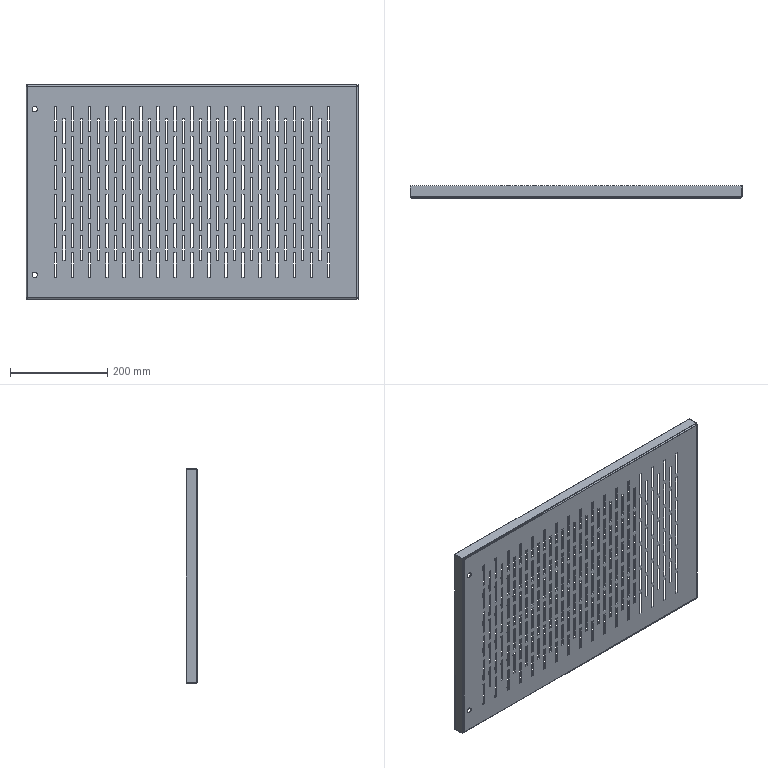Part | STEP file | 1 solid | 794 faces | box 682 x 24 x 440 mm | volume 453333 mm3 | plane 766 | cylinder 28 | commonest cylinder face diameters 7 x16 3 x4 6 x4 11 x4